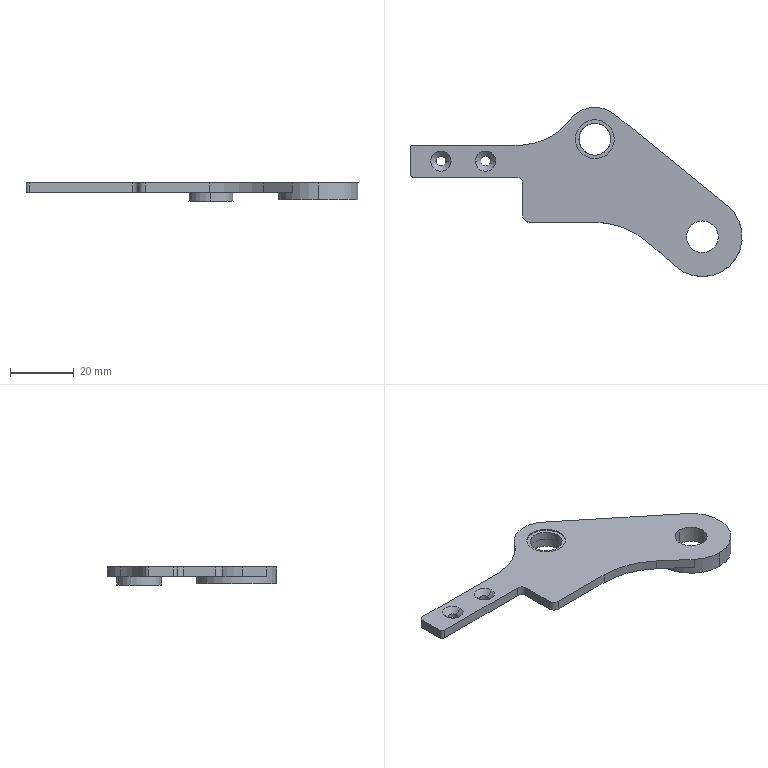Part | NX | features BREP 2, Delete Body 1 | 1 solid | 39 faces | box 104.242 x 53.12 x 5.7 mm | volume 7724 mm3 | cylinder 22 | plane 12 | cone 4 | spline 1 | commonest cylinder face diameters 10 x6 3 x4 2 x2 4 x2 12.2 x2 14 x2
STEP:
#1=CARTESIAN_POINT('',(-175.404,191.172,-0.7));
#2=VERTEX_POINT('',#1);
#3=CARTESIAN_POINT('',(-175.404,201.172,-0.7));
#4=VERTEX_POINT('',#3);
#5=CARTESIAN_POINT('',(-175.404,196.172,-0.7));
#6=DIRECTION('',(0.,0.,-1.));
#7=DIRECTION('',(0.,1.,0.));
#8=AXIS2_PLACEMENT_3D('',#5,#6,#7);
#9=CIRCLE('',#8,5.);
#10=EDGE_CURVE('',#2,#4,#9,.T.);
#11=ORIENTED_EDGE('',*,*,#10,.T.);
#12=CARTESIAN_POINT('',(-175.404,201.172,2.));
#13=VERTEX_POINT('',#12);
#14=CARTESIAN_POINT('',(-175.404,201.172,-17.671));
#15=DIRECTION('',(0.,0.,1.));
#16=VECTOR('',#15,1000.);
#17=LINE('',#14,#16);
#18=EDGE_CURVE('',#13,#4,#17,.F.);
#19=ORIENTED_EDGE('',*,*,#18,.F.);
#20=CARTESIAN_POINT('',(-176.152,201.116,2.));
#21=VERTEX_POINT('',#20);
#22=CARTESIAN_POINT('',(-175.404,201.172,2.));
#23=CARTESIAN_POINT('',(-175.654,201.172,2.));
#24=CARTESIAN_POINT('',(-175.904,201.153,2.));
#25=CARTESIAN_POINT('',(-176.152,201.116,2.));
#26=B_SPLINE_CURVE_WITH_KNOTS('',3,(#22,#23,#24,#25),.UNSPECIFIED.,.F.,.F.,(4,4),(0.,1.),.UNSPECIFIED.);
#27=EDGE_CURVE('',#21,#13,#26,.F.);
#28=ORIENTED_EDGE('',*,*,#27,.F.);
#29=CARTESIAN_POINT('',(-180.403,196.114,2.));
#30=VERTEX_POINT('',#29);
#31=CARTESIAN_POINT('',(-176.152,201.116,2.));
#32=CARTESIAN_POINT('',(-177.332,200.937,2.));
#33=CARTESIAN_POINT('',(-179.552,199.698,2.));
#34=CARTESIAN_POINT('',(-180.417,197.307,2.));
#35=CARTESIAN_POINT('',(-180.403,196.114,2.));
#36=B_SPLINE_CURVE_WITH_KNOTS('',3,(#31,#32,#33,#34,#35),.UNSPECIFIED.,.F.,.F.,(4,1,4),(0.,0.5,1.),.UNSPECIFIED.);
#37=EDGE_CURVE('',#30,#21,#36,.F.);
#38=ORIENTED_EDGE('',*,*,#37,.F.);
#39=CARTESIAN_POINT('',(-175.404,191.172,2.));
#40=VERTEX_POINT('',#39);
#41=CARTESIAN_POINT('',(-180.403,196.114,2.));
#42=CARTESIAN_POINT('',(-180.388,194.815,2.));
#43=CARTESIAN_POINT('',(-179.292,192.239,2.));
#44=CARTESIAN_POINT('',(-176.703,191.172,2.));
#45=CARTESIAN_POINT('',(-175.404,191.172,2.));
#46=B_SPLINE_CURVE_WITH_KNOTS('',3,(#41,#42,#43,#44,#45),.UNSPECIFIED.,.F.,.F.,(4,1,4),(0.,0.5,1.),.UNSPECIFIED.);
#47=EDGE_CURVE('',#40,#30,#46,.F.);
#48=ORIENTED_EDGE('',*,*,#47,.F.);
#49=CARTESIAN_POINT('',(-175.404,191.172,-17.671));
#50=DIRECTION('',(0.,0.,1.));
#51=VECTOR('',#50,1000.);
#52=LINE('',#49,#51);
#53=EDGE_CURVE('',#40,#2,#52,.F.);
#54=ORIENTED_EDGE('',*,*,#53,.T.);
#55=EDGE_LOOP('',(#11,#19,#28,#38,#48,#54));
#56=FACE_BOUND('',#55,.T.);
#57=CARTESIAN_POINT('',(-175.404,196.172,-17.671));
#58=DIRECTION('',(0.,0.,1.));
#59=DIRECTION('',(0.,1.,0.));
#60=AXIS2_PLACEMENT_3D('',#57,#58,#59);
#61=CYLINDRICAL_SURFACE('',#60,5.);
#62=ADVANCED_FACE('',(#56),#61,.F.);
#63=CARTESIAN_POINT('',(-175.404,203.172,-0.7));
#64=VERTEX_POINT('',#63);
#65=CARTESIAN_POINT('',(-175.404,189.172,-0.7));
#66=VERTEX_POINT('',#65);
#67=CARTESIAN_POINT('',(-175.404,196.172,-0.7));
#68=DIRECTION('',(0.,0.,-1.));
#69=DIRECTION('',(0.,1.,0.));
#70=AXIS2_PLACEMENT_3D('',#67,#68,#69);
#71=CIRCLE('',#70,7.);
#72=EDGE_CURVE('',#64,#66,#71,.T.);
#73=ORIENTED_EDGE('',*,*,#72,.F.);
#74=CARTESIAN_POINT('',(-175.404,203.172,2.));
#75=VERTEX_POINT('',#74);
#76=CARTESIAN_POINT('',(-175.404,203.172,-17.671));
#77=DIRECTION('',(0.,0.,1.));
#78=VECTOR('',#77,1000.);
#79=LINE('',#76,#78);
#80=EDGE_CURVE('',#75,#64,#79,.F.);
#81=ORIENTED_EDGE('',*,*,#80,.F.);
#82=CARTESIAN_POINT('',(-175.404,189.172,2.));
#83=VERTEX_POINT('',#82);
#84=CARTESIAN_POINT('',(-175.404,196.172,2.));
#85=DIRECTION('',(0.,0.,-1.));
#86=DIRECTION('',(0.,1.,0.));
#87=AXIS2_PLACEMENT_3D('',#84,#85,#86);
#88=CIRCLE('',#87,7.);
#89=EDGE_CURVE('',#75,#83,#88,.T.);
#90=ORIENTED_EDGE('',*,*,#89,.T.);
#91=CARTESIAN_POINT('',(-175.404,189.172,-17.671));
#92=DIRECTION('',(0.,0.,1.));
#93=VECTOR('',#92,1000.);
#94=LINE('',#91,#93);
#95=EDGE_CURVE('',#83,#66,#94,.F.);
#96=ORIENTED_EDGE('',*,*,#95,.T.);
#97=EDGE_LOOP('',(#73,#81,#90,#96));
#98=FACE_BOUND('',#97,.T.);
#99=CARTESIAN_POINT('',(-175.404,196.172,-17.671));
#100=DIRECTION('',(0.,0.,1.));
#101=DIRECTION('',(0.,1.,0.));
#102=AXIS2_PLACEMENT_3D('',#99,#100,#101);
#103=CYLINDRICAL_SURFACE('',#102,7.);
#104=ADVANCED_FACE('',(#98),#103,.T.);
#105=CARTESIAN_POINT('',(-141.672,178.052,-0.3));
#106=VERTEX_POINT('',#105);
#107=CARTESIAN_POINT('',(-141.672,153.052,-0.3));
#108=VERTEX_POINT('',#107);
#109=CARTESIAN_POINT('',(-141.672,165.552,-0.3));
#110=DIRECTION('',(0.,0.,-1.));
#111=DIRECTION('',(0.,1.,0.));
#112=AXIS2_PLACEMENT_3D('',#109,#110,#111);
#113=CIRCLE('',#112,12.5);
#114=EDGE_CURVE('',#106,#108,#113,.T.);
#115=ORIENTED_EDGE('',*,*,#114,.F.);
#116=CARTESIAN_POINT('',(-141.672,178.052,2.));
#117=VERTEX_POINT('',#116);
#118=CARTESIAN_POINT('',(-141.672,178.052,2.));
#119=DIRECTION('',(0.,0.,1.));
#120=VECTOR('',#119,1000.);
#121=LINE('',#118,#120);
#122=EDGE_CURVE('',#117,#106,#121,.F.);
#123=ORIENTED_EDGE('',*,*,#122,.F.);
#124=CARTESIAN_POINT('',(-133.791,175.255,2.));
#125=VERTEX_POINT('',#124);
#126=CARTESIAN_POINT('',(-141.672,165.552,2.));
#127=DIRECTION('',(0.,0.,-1.));
#128=DIRECTION('',(0.,1.,0.));
#129=AXIS2_PLACEMENT_3D('',#126,#127,#128);
#130=CIRCLE('',#129,12.5);
#131=EDGE_CURVE('',#117,#125,#130,.T.);
#132=ORIENTED_EDGE('',*,*,#131,.T.);
#133=CARTESIAN_POINT('',(-133.791,175.255,5.));
#134=VERTEX_POINT('',#133);
#135=CARTESIAN_POINT('',(-133.791,175.255,2.));
#136=DIRECTION('',(0.,0.,1.));
#137=VECTOR('',#136,1000.);
#138=LINE('',#135,#137);
#139=EDGE_CURVE('',#125,#134,#138,.T.);
#140=ORIENTED_EDGE('',*,*,#139,.T.);
#141=CARTESIAN_POINT('',(-141.672,153.052,5.));
#142=VERTEX_POINT('',#141);
#143=CARTESIAN_POINT('',(-141.672,165.552,5.));
#144=DIRECTION('',(0.,0.,-1.));
#145=DIRECTION('',(0.,1.,0.));
#146=AXIS2_PLACEMENT_3D('',#143,#144,#145);
#147=CIRCLE('',#146,12.5);
#148=EDGE_CURVE('',#134,#142,#147,.T.);
#149=ORIENTED_EDGE('',*,*,#148,.T.);
#150=CARTESIAN_POINT('',(-141.672,153.052,2.));
#151=DIRECTION('',(0.,0.,1.));
#152=VECTOR('',#151,1000.);
#153=LINE('',#150,#152);
#154=EDGE_CURVE('',#142,#108,#153,.F.);
#155=ORIENTED_EDGE('',*,*,#154,.T.);
#156=EDGE_LOOP('',(#115,#123,#132,#140,#149,#155));
#157=FACE_BOUND('',#156,.T.);
#158=CARTESIAN_POINT('',(-141.672,165.552,2.));
#159=DIRECTION('',(0.,0.,1.));
#160=DIRECTION('',(0.,1.,0.));
#161=AXIS2_PLACEMENT_3D('',#158,#159,#160);
#162=CYLINDRICAL_SURFACE('',#161,12.5);
#163=ADVANCED_FACE('',(#157),#162,.T.);
#164=CARTESIAN_POINT('',(-208.209,189.293,2.));
#165=VERTEX_POINT('',#164);
#166=CARTESIAN_POINT('',(-211.209,189.293,2.));
#167=VERTEX_POINT('',#166);
#168=CARTESIAN_POINT('',(-209.709,189.293,2.));
#169=DIRECTION('',(0.,0.,-1.));
#170=DIRECTION('',(0.,1.,0.));
#171=AXIS2_PLACEMENT_3D('',#168,#169,#170);
#172=CIRCLE('',#171,1.5);
#173=EDGE_CURVE('',#165,#167,#172,.T.);
#174=ORIENTED_EDGE('',*,*,#173,.T.);
#175=CARTESIAN_POINT('',(-211.209,189.293,3.3));
#176=VERTEX_POINT('',#175);
#177=CARTESIAN_POINT('',(-211.209,189.293,-0.5));
#178=DIRECTION('',(0.,0.,1.));
#179=VECTOR('',#178,1000.);
#180=LINE('',#177,#179);
#181=EDGE_CURVE('',#167,#176,#180,.T.);
#182=ORIENTED_EDGE('',*,*,#181,.T.);
#183=CARTESIAN_POINT('',(-208.209,189.293,3.3));
#184=VERTEX_POINT('',#183);
#185=CARTESIAN_POINT('',(-209.709,189.293,3.3));
#186=DIRECTION('',(0.,0.,1.));
#187=DIRECTION('',(-1.,0.,0.));
#188=AXIS2_PLACEMENT_3D('',#185,#186,#187);
#189=CIRCLE('',#188,1.5);
#190=EDGE_CURVE('',#176,#184,#189,.T.);
#191=ORIENTED_EDGE('',*,*,#190,.T.);
#192=CARTESIAN_POINT('',(-208.209,189.293,-0.5));
#193=DIRECTION('',(0.,0.,1.));
#194=VECTOR('',#193,1000.);
#195=LINE('',#192,#194);
#196=EDGE_CURVE('',#165,#184,#195,.T.);
#197=ORIENTED_EDGE('',*,*,#196,.F.);
#198=EDGE_LOOP('',(#174,#182,#191,#197));
#199=FACE_BOUND('',#198,.T.);
#200=CARTESIAN_POINT('',(-209.709,189.293,-0.5));
#201=DIRECTION('',(0.,0.,1.));
#202=DIRECTION('',(-1.,0.,0.));
#203=AXIS2_PLACEMENT_3D('',#200,#201,#202);
#204=CYLINDRICAL_SURFACE('',#203,1.5);
#205=ADVANCED_FACE('',(#199),#204,.F.);
#206=CARTESIAN_POINT('',(-222.209,189.293,2.));
#207=VERTEX_POINT('',#206);
#208=CARTESIAN_POINT('',(-225.209,189.293,2.));
#209=VERTEX_POINT('',#208);
#210=CARTESIAN_POINT('',(-223.709,189.293,2.));
#211=DIRECTION('',(0.,0.,-1.));
#212=DIRECTION('',(0.,1.,0.));
#213=AXIS2_PLACEMENT_3D('',#210,#211,#212);
#214=CIRCLE('',#213,1.5);
#215=EDGE_CURVE('',#207,#209,#214,.T.);
#216=ORIENTED_EDGE('',*,*,#215,.T.);
#217=CARTESIAN_POINT('',(-225.209,189.293,3.3));
#218=VERTEX_POINT('',#217);
#219=CARTESIAN_POINT('',(-225.209,189.293,-0.5));
#220=DIRECTION('',(0.,0.,1.));
#221=VECTOR('',#220,1000.);
#222=LINE('',#219,#221);
#223=EDGE_CURVE('',#209,#218,#222,.T.);
#224=ORIENTED_EDGE('',*,*,#223,.T.);
#225=CARTESIAN_POINT('',(-222.209,189.293,3.3));
#226=VERTEX_POINT('',#225);
#227=CARTESIAN_POINT('',(-223.709,189.293,3.3));
#228=DIRECTION('',(0.,0.,1.));
#229=DIRECTION('',(-1.,0.,0.));
#230=AXIS2_PLACEMENT_3D('',#227,#228,#229);
#231=CIRCLE('',#230,1.5);
#232=EDGE_CURVE('',#218,#226,#231,.T.);
#233=ORIENTED_EDGE('',*,*,#232,.T.);
#234=CARTESIAN_POINT('',(-222.209,189.293,-0.5));
#235=DIRECTION('',(0.,0.,1.));
#236=VECTOR('',#235,1000.);
#237=LINE('',#234,#236);
#238=EDGE_CURVE('',#207,#226,#237,.T.);
#239=ORIENTED_EDGE('',*,*,#238,.F.);
#240=EDGE_LOOP('',(#216,#224,#233,#239));
#241=FACE_BOUND('',#240,.T.);
#242=CARTESIAN_POINT('',(-223.709,189.293,-0.5));
#243=DIRECTION('',(0.,0.,1.));
#244=DIRECTION('',(-1.,0.,0.));
#245=AXIS2_PLACEMENT_3D('',#242,#243,#244);
#246=CYLINDRICAL_SURFACE('',#245,1.5);
#247=ADVANCED_FACE('',(#241),#246,.F.);
#248=CARTESIAN_POINT('',(-181.503,196.101,5.));
#249=VERTEX_POINT('',#248);
#250=CARTESIAN_POINT('',(-169.304,196.243,5.));
#251=VERTEX_POINT('',#250);
#252=CARTESIAN_POINT('',(-175.403,196.172,5.));
#253=DIRECTION('',(0.,0.,1.));
#254=DIRECTION('',(0.,1.,0.));
#255=AXIS2_PLACEMENT_3D('',#252,#253,#254);
#256=CIRCLE('',#255,6.1);
#257=EDGE_CURVE('',#249,#251,#256,.T.);
#258=ORIENTED_EDGE('',*,*,#257,.T.);
#259=CARTESIAN_POINT('',(-169.304,196.243,4.6));
#260=VERTEX_POINT('',#259);
#261=CARTESIAN_POINT('',(-169.304,196.243,2.785));
#262=DIRECTION('',(0.,0.,-1.));
#263=VECTOR('',#262,1000.);
#264=LINE('',#261,#263);
#265=EDGE_CURVE('',#260,#251,#264,.F.);
#266=ORIENTED_EDGE('',*,*,#265,.F.);
#267=CARTESIAN_POINT('',(-181.503,196.101,4.6));
#268=VERTEX_POINT('',#267);
#269=CARTESIAN_POINT('',(-175.403,196.172,4.6));
#270=DIRECTION('',(0.,0.,-1.));
#271=DIRECTION('',(0.,-1.,0.));
#272=AXIS2_PLACEMENT_3D('',#269,#270,#271);
#273=CIRCLE('',#272,6.1);
#274=EDGE_CURVE('',#260,#268,#273,.T.);
#275=ORIENTED_EDGE('',*,*,#274,.T.);
#276=CARTESIAN_POINT('',(-181.503,196.101,2.785));
#277=DIRECTION('',(0.,0.,-1.));
#278=VECTOR('',#277,1000.);
#279=LINE('',#276,#278);
#280=EDGE_CURVE('',#268,#249,#279,.F.);
#281=ORIENTED_EDGE('',*,*,#280,.T.);
#282=EDGE_LOOP('',(#258,#266,#275,#281));
#283=FACE_BOUND('',#282,.T.);
#284=CARTESIAN_POINT('',(-175.403,196.172,2.785));
#285=DIRECTION('',(0.,0.,-1.));
#286=DIRECTION('',(0.9999,0.01167,0.));
#287=AXIS2_PLACEMENT_3D('',#284,#285,#286);
#288=CYLINDRICAL_SURFACE('',#287,6.1);
#289=ADVANCED_FACE('',(#283),#288,.F.);
#290=ORIENTED_EDGE('',*,*,#190,.F.);
#291=CARTESIAN_POINT('',(-212.909,189.293,5.));
#292=VERTEX_POINT('',#291);
#293=CARTESIAN_POINT('',(-211.209,189.293,3.3));
#294=DIRECTION('',(-0.7071,0.,0.7071));
#295=VECTOR('',#294,1000.);
#296=LINE('',#293,#295);
#297=EDGE_CURVE('',#176,#292,#296,.T.);
#298=ORIENTED_EDGE('',*,*,#297,.T.);
#299=CARTESIAN_POINT('',(-206.509,189.293,5.));
#300=VERTEX_POINT('',#299);
#301=CARTESIAN_POINT('',(-209.709,189.293,5.));
#302=DIRECTION('',(0.,0.,-1.));
#303=DIRECTION('',(0.,1.,0.));
#304=AXIS2_PLACEMENT_3D('',#301,#302,#303);
#305=CIRCLE('',#304,3.2);
#306=EDGE_CURVE('',#300,#292,#305,.T.);
#307=ORIENTED_EDGE('',*,*,#306,.F.);
#308=CARTESIAN_POINT('',(-208.209,189.293,3.3));
#309=DIRECTION('',(0.7071,0.,0.7071));
#310=VECTOR('',#309,1000.);
#311=LINE('',#308,#310);
#312=EDGE_CURVE('',#184,#300,#311,.T.);
#313=ORIENTED_EDGE('',*,*,#312,.F.);
#314=EDGE_LOOP('',(#290,#298,#307,#313));
#315=FACE_BOUND('',#314,.T.);
#316=CARTESIAN_POINT('',(-209.709,189.293,3.3));
#317=DIRECTION('',(0.,0.,1.));
#318=DIRECTION('',(-1.,0.,0.));
#319=AXIS2_PLACEMENT_3D('',#316,#317,#318);
#320=CONICAL_SURFACE('',#319,1.5,0.7854);
#321=ADVANCED_FACE('',(#315),#320,.F.);
#322=ORIENTED_EDGE('',*,*,#232,.F.);
#323=CARTESIAN_POINT('',(-226.909,189.293,5.));
#324=VERTEX_POINT('',#323);
#325=CARTESIAN_POINT('',(-225.209,189.293,3.3));
#326=DIRECTION('',(-0.7071,0.,0.7071));
#327=VECTOR('',#326,1000.);
#328=LINE('',#325,#327);
#329=EDGE_CURVE('',#218,#324,#328,.T.);
#330=ORIENTED_EDGE('',*,*,#329,.T.);
#331=CARTESIAN_POINT('',(-220.509,189.293,5.));
#332=VERTEX_POINT('',#331);
#333=CARTESIAN_POINT('',(-223.709,189.293,5.));
#334=DIRECTION('',(0.,0.,-1.));
#335=DIRECTION('',(0.,1.,0.));
#336=AXIS2_PLACEMENT_3D('',#333,#334,#335);
#337=CIRCLE('',#336,3.2);
#338=EDGE_CURVE('',#332,#324,#337,.T.);
#339=ORIENTED_EDGE('',*,*,#338,.F.);
#340=CARTESIAN_POINT('',(-222.209,189.293,3.3));
#341=DIRECTION('',(0.7071,0.,0.7071));
#342=VECTOR('',#341,1000.);
#343=LINE('',#340,#342);
#344=EDGE_CURVE('',#226,#332,#343,.T.);
#345=ORIENTED_EDGE('',*,*,#344,.F.);
#346=EDGE_LOOP('',(#322,#330,#339,#345));
#347=FACE_BOUND('',#346,.T.);
#348=CARTESIAN_POINT('',(-223.709,189.293,3.3));
#349=DIRECTION('',(0.,0.,1.));
#350=DIRECTION('',(-1.,0.,0.));
#351=AXIS2_PLACEMENT_3D('',#348,#349,#350);
#352=CONICAL_SURFACE('',#351,1.5,0.7854);
#353=ADVANCED_FACE('',(#347),#352,.F.);
#354=CARTESIAN_POINT('',(-141.672,160.552,-0.3));
#355=VERTEX_POINT('',#354);
#356=CARTESIAN_POINT('',(-141.672,170.552,-0.3));
#357=VERTEX_POINT('',#356);
#358=CARTESIAN_POINT('',(-141.672,165.552,-0.3));
#359=DIRECTION('',(0.,0.,-1.));
#360=DIRECTION('',(0.,1.,0.));
#361=AXIS2_PLACEMENT_3D('',#358,#359,#360);
#362=CIRCLE('',#361,5.);
#363=EDGE_CURVE('',#355,#357,#362,.T.);
#364=ORIENTED_EDGE('',*,*,#363,.T.);
#365=CARTESIAN_POINT('',(-141.672,170.552,5.));
#366=VERTEX_POINT('',#365);
#367=CARTESIAN_POINT('',(-141.672,170.552,2.));
#368=DIRECTION('',(0.,0.,1.));
#369=VECTOR('',#368,1000.);
#370=LINE('',#367,#369);
#371=EDGE_CURVE('',#366,#357,#370,.F.);
#372=ORIENTED_EDGE('',*,*,#371,.F.);
#373=CARTESIAN_POINT('',(-141.672,160.552,5.));
#374=VERTEX_POINT('',#373);
#375=CARTESIAN_POINT('',(-141.672,165.552,5.));
#376=DIRECTION('',(0.,0.,-1.));
#377=DIRECTION('',(0.,1.,0.));
#378=AXIS2_PLACEMENT_3D('',#375,#376,#377);
#379=CIRCLE('',#378,5.);
#380=EDGE_CURVE('',#374,#366,#379,.T.);
#381=ORIENTED_EDGE('',*,*,#380,.F.);
#382=CARTESIAN_POINT('',(-141.672,160.552,2.));
#383=DIRECTION('',(0.,0.,1.));
#384=VECTOR('',#383,1000.);
#385=LINE('',#382,#384);
#386=EDGE_CURVE('',#374,#355,#385,.F.);
#387=ORIENTED_EDGE('',*,*,#386,.T.);
#388=EDGE_LOOP('',(#364,#372,#381,#387));
#389=FACE_BOUND('',#388,.T.);
#390=CARTESIAN_POINT('',(-141.672,165.552,2.));
#391=DIRECTION('',(0.,0.,1.));
#392=DIRECTION('',(0.,1.,0.));
#393=AXIS2_PLACEMENT_3D('',#390,#391,#392);
#394=CYLINDRICAL_SURFACE('',#393,5.);
#395=ADVANCED_FACE('',(#389),#394,.F.);
#396=CARTESIAN_POINT('',(-180.403,196.114,4.6));
#397=VERTEX_POINT('',#396);
#398=CARTESIAN_POINT('',(-170.403,196.231,4.6));
#399=VERTEX_POINT('',#398);
#400=CARTESIAN_POINT('',(-175.403,196.172,4.6));
#401=DIRECTION('',(0.,0.,1.));
#402=DIRECTION('',(0.,-1.,0.));
#403=AXIS2_PLACEMENT_3D('',#400,#401,#402);
#404=CIRCLE('',#403,5.);
#405=EDGE_CURVE('',#397,#399,#404,.T.);
#406=ORIENTED_EDGE('',*,*,#405,.T.);
#407=CARTESIAN_POINT('',(-170.404,196.231,2.));
#408=VERTEX_POINT('',#407);
#409=CARTESIAN_POINT('',(-170.403,196.231,2.785));
#410=DIRECTION('',(0.,0.,-1.));
#411=VECTOR('',#410,1000.);
#412=LINE('',#409,#411);
#413=EDGE_CURVE('',#408,#399,#412,.F.);
#414=ORIENTED_EDGE('',*,*,#413,.F.);
#415=CARTESIAN_POINT('',(-174.655,191.228,2.));
#416=VERTEX_POINT('',#415);
#417=CARTESIAN_POINT('',(-170.403,196.231,2.));
#418=CARTESIAN_POINT('',(-170.39,195.037,2.));
#419=CARTESIAN_POINT('',(-171.254,192.646,2.));
#420=CARTESIAN_POINT('',(-173.475,191.407,2.));
#421=CARTESIAN_POINT('',(-174.655,191.228,2.));
#422=B_SPLINE_CURVE_WITH_KNOTS('',3,(#417,#418,#419,#420,#421),.UNSPECIFIED.,.F.,.F.,(4,1,4),(0.,0.5,1.),.UNSPECIFIED.);
#423=EDGE_CURVE('',#408,#416,#422,.T.);
#424=ORIENTED_EDGE('',*,*,#423,.T.);
#425=CARTESIAN_POINT('',(-174.655,191.228,2.));
#426=CARTESIAN_POINT('',(-174.903,191.191,2.));
#427=CARTESIAN_POINT('',(-175.153,191.172,2.));
#428=CARTESIAN_POINT('',(-175.404,191.172,2.));
#429=B_SPLINE_CURVE_WITH_KNOTS('',3,(#425,#426,#427,#428),.UNSPECIFIED.,.F.,.F.,(4,4),(0.,1.),.UNSPECIFIED.);
#430=EDGE_CURVE('',#416,#40,#429,.T.);
#431=ORIENTED_EDGE('',*,*,#430,.T.);
#432=ORIENTED_EDGE('',*,*,#47,.T.);
#433=CARTESIAN_POINT('',(-180.403,196.114,2.785));
#434=DIRECTION('',(0.,0.,-1.));
#435=VECTOR('',#434,1000.);
#436=LINE('',#433,#435);
#437=EDGE_CURVE('',#30,#397,#436,.F.);
#438=ORIENTED_EDGE('',*,*,#437,.T.);
#439=EDGE_LOOP('',(#406,#414,#424,#431,#432,#438));
#440=FACE_BOUND('',#439,.T.);
#441=CARTESIAN_POINT('',(-175.403,196.172,2.785));
#442=DIRECTION('',(0.,0.,-1.));
#443=DIRECTION('',(0.9999,0.01167,0.));
#444=AXIS2_PLACEMENT_3D('',#441,#442,#443);
#445=CYLINDRICAL_SURFACE('',#444,5.);
#446=ADVANCED_FACE('',(#440),#445,.F.);
#447=ORIENTED_EDGE('',*,*,#413,.T.);
#448=CARTESIAN_POINT('',(-175.403,196.172,4.6));
#449=DIRECTION('',(0.,0.,1.));
#450=DIRECTION('',(0.,-1.,0.));
#451=AXIS2_PLACEMENT_3D('',#448,#449,#450);
#452=CIRCLE('',#451,5.);
#453=EDGE_CURVE('',#399,#397,#452,.T.);
#454=ORIENTED_EDGE('',*,*,#453,.T.);
#455=ORIENTED_EDGE('',*,*,#437,.F.);
#456=ORIENTED_EDGE('',*,*,#37,.T.);
#457=ORIENTED_EDGE('',*,*,#27,.T.);
#458=CARTESIAN_POINT('',(-175.404,201.172,2.));
#459=CARTESIAN_POINT('',(-174.104,201.172,2.));
#460=CARTESIAN_POINT('',(-171.515,200.106,2.));
#461=CARTESIAN_POINT('',(-170.419,197.53,2.));
#462=CARTESIAN_POINT('',(-170.403,196.231,2.));
#463=B_SPLINE_CURVE_WITH_KNOTS('',3,(#458,#459,#460,#461,#462),.UNSPECIFIED.,.F.,.F.,(4,1,4),(0.,0.5,1.),.UNSPECIFIED.);
#464=EDGE_CURVE('',#13,#408,#463,.T.);
#465=ORIENTED_EDGE('',*,*,#464,.T.);
#466=EDGE_LOOP('',(#447,#454,#455,#456,#457,#465));
#467=FACE_BOUND('',#466,.T.);
#468=CARTESIAN_POINT('',(-175.403,196.172,2.785));
#469=DIRECTION('',(0.,0.,-1.));
#470=DIRECTION('',(0.9999,0.01167,0.));
#471=AXIS2_PLACEMENT_3D('',#468,#469,#470);
#472=CYLINDRICAL_SURFACE('',#471,5.);
#473=ADVANCED_FACE('',(#467),#472,.F.);
#474=ORIENTED_EDGE('',*,*,#371,.T.);
#475=CARTESIAN_POINT('',(-141.672,165.552,-0.3));
#476=DIRECTION('',(0.,0.,-1.));
#477=DIRECTION('',(0.,1.,0.));
#478=AXIS2_PLACEMENT_3D('',#475,#476,#477);
#479=CIRCLE('',#478,5.);
#480=EDGE_CURVE('',#357,#355,#479,.T.);
#481=ORIENTED_EDGE('',*,*,#480,.T.);
#482=ORIENTED_EDGE('',*,*,#386,.F.);
#483=CARTESIAN_POINT('',(-141.672,165.552,5.));
#484=DIRECTION('',(0.,0.,-1.));
#485=DIRECTION('',(0.,1.,0.));
#486=AXIS2_PLACEMENT_3D('',#483,#484,#485);
#487=CIRCLE('',#486,5.);
#488=EDGE_CURVE('',#366,#374,#487,.T.);
#489=ORIENTED_EDGE('',*,*,#488,.F.);
#490=EDGE_LOOP('',(#474,#481,#482,#489));
#491=FACE_BOUND('',#490,.T.);
#492=CARTESIAN_POINT('',(-141.672,165.552,2.));
#493=DIRECTION('',(0.,0.,1.));
#494=DIRECTION('',(0.,1.,0.));
#495=AXIS2_PLACEMENT_3D('',#492,#493,#494);
#496=CYLINDRICAL_SURFACE('',#495,5.);
#497=ADVANCED_FACE('',(#491),#496,.F.);
#498=ORIENTED_EDGE('',*,*,#329,.F.);
#499=CARTESIAN_POINT('',(-223.709,189.293,3.3));
#500=DIRECTION('',(0.,0.,1.));
#501=DIRECTION('',(-1.,0.,0.));
#502=AXIS2_PLACEMENT_3D('',#499,#500,#501);
#503=CIRCLE('',#502,1.5);
#504=EDGE_CURVE('',#226,#218,#503,.T.);
#505=ORIENTED_EDGE('',*,*,#504,.F.);
#506=ORIENTED_EDGE('',*,*,#344,.T.);
#507=CARTESIAN_POINT('',(-223.709,189.293,5.));
#508=DIRECTION('',(0.,0.,-1.));
#509=DIRECTION('',(0.,1.,0.));
#510=AXIS2_PLACEMENT_3D('',#507,#508,#509);
#511=CIRCLE('',#510,3.2);
#512=EDGE_CURVE('',#324,#332,#511,.T.);
#513=ORIENTED_EDGE('',*,*,#512,.F.);
#514=EDGE_LOOP('',(#498,#505,#506,#513));
#515=FACE_BOUND('',#514,.T.);
#516=CARTESIAN_POINT('',(-223.709,189.293,3.3));
#517=DIRECTION('',(0.,0.,1.));
#518=DIRECTION('',(-1.,0.,0.));
#519=AXIS2_PLACEMENT_3D('',#516,#517,#518);
#520=CONICAL_SURFACE('',#519,1.5,0.7854);
#521=ADVANCED_FACE('',(#515),#520,.F.);
#522=ORIENTED_EDGE('',*,*,#297,.F.);
#523=CARTESIAN_POINT('',(-209.709,189.293,3.3));
#524=DIRECTION('',(0.,0.,1.));
#525=DIRECTION('',(-1.,0.,0.));
#526=AXIS2_PLACEMENT_3D('',#523,#524,#525);
#527=CIRCLE('',#526,1.5);
#528=EDGE_CURVE('',#184,#176,#527,.T.);
#529=ORIENTED_EDGE('',*,*,#528,.F.);
#530=ORIENTED_EDGE('',*,*,#312,.T.);
#531=CARTESIAN_POINT('',(-209.709,189.293,5.));
#532=DIRECTION('',(0.,0.,-1.));
#533=DIRECTION('',(0.,1.,0.));
#534=AXIS2_PLACEMENT_3D('',#531,#532,#533);
#535=CIRCLE('',#534,3.2);
#536=EDGE_CURVE('',#292,#300,#535,.T.);
#537=ORIENTED_EDGE('',*,*,#536,.F.);
#538=EDGE_LOOP('',(#522,#529,#530,#537));
#539=FACE_BOUND('',#538,.T.);
#540=CARTESIAN_POINT('',(-209.709,189.293,3.3));
#541=DIRECTION('',(0.,0.,1.));
#542=DIRECTION('',(-1.,0.,0.));
#543=AXIS2_PLACEMENT_3D('',#540,#541,#542);
#544=CONICAL_SURFACE('',#543,1.5,0.7854);
#545=ADVANCED_FACE('',(#539),#544,.F.);
#546=CARTESIAN_POINT('',(-141.672,165.552,-0.3));
#547=DIRECTION('',(0.,0.,-1.));
#548=DIRECTION('',(0.,1.,0.));
#549=AXIS2_PLACEMENT_3D('',#546,#547,#548);
#550=CIRCLE('',#549,12.5);
#551=EDGE_CURVE('',#108,#106,#550,.T.);
#552=ORIENTED_EDGE('',*,*,#551,.T.);
#553=ORIENTED_EDGE('',*,*,#114,.T.);
#554=EDGE_LOOP('',(#552,#553));
#555=FACE_BOUND('',#554,.T.);
#556=ORIENTED_EDGE('',*,*,#363,.F.);
#557=ORIENTED_EDGE('',*,*,#480,.F.);
#558=EDGE_LOOP('',(#556,#557));
#559=FACE_BOUND('',#558,.T.);
#560=CARTESIAN_POINT('',(-146.593,163.872,-0.3));
#561=DIRECTION('',(0.,0.,-1.));
#562=DIRECTION('',(1.,0.,0.));
#563=AXIS2_PLACEMENT_3D('',#560,#561,#562);
#564=PLANE('',#563);
#565=ADVANCED_FACE('',(#555,#559),#564,.T.);
#566=ORIENTED_EDGE('',*,*,#265,.T.);
#567=CARTESIAN_POINT('',(-175.403,196.172,5.));
#568=DIRECTION('',(0.,0.,1.));
#569=DIRECTION('',(0.,1.,0.));
#570=AXIS2_PLACEMENT_3D('',#567,#568,#569);
#571=CIRCLE('',#570,6.1);
#572=EDGE_CURVE('',#251,#249,#571,.T.);
#573=ORIENTED_EDGE('',*,*,#572,.T.);
#574=ORIENTED_EDGE('',*,*,#280,.F.);
#575=CARTESIAN_POINT('',(-175.403,196.172,4.6));
#576=DIRECTION('',(0.,0.,-1.));
#577=DIRECTION('',(0.,-1.,0.));
#578=AXIS2_PLACEMENT_3D('',#575,#576,#577);
#579=CIRCLE('',#578,6.1);
#580=EDGE_CURVE('',#268,#260,#579,.T.);
#581=ORIENTED_EDGE('',*,*,#580,.T.);
#582=EDGE_LOOP('',(#566,#573,#574,#581));
#583=FACE_BOUND('',#582,.T.);
#584=CARTESIAN_POINT('',(-175.403,196.172,2.785));
#585=DIRECTION('',(0.,0.,-1.));
#586=DIRECTION('',(0.9999,0.01167,0.));
#587=AXIS2_PLACEMENT_3D('',#584,#585,#586);
#588=CYLINDRICAL_SURFACE('',#587,6.1);
#589=ADVANCED_FACE('',(#583),#588,.F.);
#590=ORIENTED_EDGE('',*,*,#580,.F.);
#591=ORIENTED_EDGE('',*,*,#274,.F.);
#592=EDGE_LOOP('',(#590,#591));
#593=FACE_BOUND('',#592,.T.);
#594=ORIENTED_EDGE('',*,*,#405,.F.);
#595=ORIENTED_EDGE('',*,*,#453,.F.);
#596=EDGE_LOOP('',(#594,#595));
#597=FACE_BOUND('',#596,.T.);
#598=CARTESIAN_POINT('',(-175.464,201.372,4.6));
#599=DIRECTION('',(0.,0.,1.));
#600=DIRECTION('',(-1.,0.,0.));
#601=AXIS2_PLACEMENT_3D('',#598,#599,#600);
#602=PLANE('',#601);
#603=ADVANCED_FACE('',(#593,#597),#602,.T.);
#604=CARTESIAN_POINT('',(-169.098,203.934,5.));
#605=VERTEX_POINT('',#604);
#606=CARTESIAN_POINT('',(32.582,40.112,5.));
#607=DIRECTION('',(-0.7762,0.6305,0.));
#608=VECTOR('',#607,1000.);
#609=LINE('',#606,#608);
#610=EDGE_CURVE('',#134,#605,#609,.T.);
#611=ORIENTED_EDGE('',*,*,#610,.T.);
#612=CARTESIAN_POINT('',(-183.399,202.177,5.));
#613=VERTEX_POINT('',#612);
#614=CARTESIAN_POINT('',(-175.403,196.172,5.));
#615=DIRECTION('',(0.,0.,1.));
#616=DIRECTION('',(1.,0.,0.));
#617=AXIS2_PLACEMENT_3D('',#614,#615,#616);
#618=CIRCLE('',#617,10.);
#619=EDGE_CURVE('',#605,#613,#618,.T.);
#620=ORIENTED_EDGE('',*,*,#619,.T.);
#621=CARTESIAN_POINT('',(-198.567,194.293,5.));
#622=VERTEX_POINT('',#621);
#623=CARTESIAN_POINT('',(-198.567,194.293,5.));
#624=CARTESIAN_POINT('',(-188.816,194.965,5.));
#625=CARTESIAN_POINT('',(-183.399,202.177,5.));
#626=B_SPLINE_CURVE_WITH_KNOTS('',2,(#623,#624,#625),.UNSPECIFIED.,.F.,.F.,(3,3),(0.,1.),.PIECEWISE_BEZIER_KNOTS.);
#627=EDGE_CURVE('',#622,#613,#626,.T.);
#628=ORIENTED_EDGE('',*,*,#627,.F.);
#629=CARTESIAN_POINT('',(-232.414,194.293,5.));
#630=VERTEX_POINT('',#629);
#631=CARTESIAN_POINT('',(-214.519,194.293,5.));
#632=DIRECTION('',(1.,0.,0.));
#633=VECTOR('',#632,1000.);
#634=LINE('',#631,#633);
#635=EDGE_CURVE('',#630,#622,#634,.T.);
#636=ORIENTED_EDGE('',*,*,#635,.F.);
#637=CARTESIAN_POINT('',(-233.414,193.293,5.));
#638=VERTEX_POINT('',#637);
#639=CARTESIAN_POINT('',(-232.414,193.293,5.));
#640=DIRECTION('',(0.,0.,1.));
#641=DIRECTION('',(0.,1.,0.));
#642=AXIS2_PLACEMENT_3D('',#639,#640,#641);
#643=CIRCLE('',#642,1.);
#644=EDGE_CURVE('',#630,#638,#643,.T.);
#645=ORIENTED_EDGE('',*,*,#644,.T.);
#646=CARTESIAN_POINT('',(-233.414,185.293,5.));
#647=VERTEX_POINT('',#646);
#648=CARTESIAN_POINT('',(-233.414,185.793,5.));
#649=DIRECTION('',(0.,-1.,0.));
#650=VECTOR('',#649,1000.);
#651=LINE('',#648,#650);
#652=EDGE_CURVE('',#638,#647,#651,.T.);
#653=ORIENTED_EDGE('',*,*,#652,.T.);
#654=CARTESIAN_POINT('',(-232.414,184.293,5.));
#655=VERTEX_POINT('',#654);
#656=CARTESIAN_POINT('',(-232.414,185.293,5.));
#657=DIRECTION('',(0.,0.,1.));
#658=DIRECTION('',(0.,1.,0.));
#659=AXIS2_PLACEMENT_3D('',#656,#657,#658);
#660=CIRCLE('',#659,1.);
#661=EDGE_CURVE('',#647,#655,#660,.T.);
#662=ORIENTED_EDGE('',*,*,#661,.T.);
#663=CARTESIAN_POINT('',(-200.068,184.293,5.));
#664=VERTEX_POINT('',#663);
#665=CARTESIAN_POINT('',(-141.672,184.293,5.));
#666=DIRECTION('',(1.,0.,0.));
#667=VECTOR('',#666,1000.);
#668=LINE('',#665,#667);
#669=EDGE_CURVE('',#655,#664,#668,.T.);
#670=ORIENTED_EDGE('',*,*,#669,.T.);
#671=CARTESIAN_POINT('',(-198.068,182.293,5.));
#672=VERTEX_POINT('',#671);
#673=CARTESIAN_POINT('',(-200.068,182.293,5.));
#674=DIRECTION('',(0.,0.,-1.));
#675=DIRECTION('',(0.,1.,0.));
#676=AXIS2_PLACEMENT_3D('',#673,#674,#675);
#677=CIRCLE('',#676,2.);
#678=EDGE_CURVE('',#664,#672,#677,.T.);
#679=ORIENTED_EDGE('',*,*,#678,.T.);
#680=CARTESIAN_POINT('',(-198.068,172.145,5.));
#681=VERTEX_POINT('',#680);
#682=CARTESIAN_POINT('',(-198.068,170.145,5.));
#683=DIRECTION('',(0.,-1.,0.));
#684=VECTOR('',#683,1000.);
#685=LINE('',#682,#684);
#686=EDGE_CURVE('',#672,#681,#685,.T.);
#687=ORIENTED_EDGE('',*,*,#686,.T.);
#688=CARTESIAN_POINT('',(-196.068,170.145,5.));
#689=VERTEX_POINT('',#688);
#690=CARTESIAN_POINT('',(-196.068,172.145,5.));
#691=DIRECTION('',(0.,0.,1.));
#692=DIRECTION('',(0.,1.,0.));
#693=AXIS2_PLACEMENT_3D('',#690,#691,#692);
#694=CIRCLE('',#693,2.);
#695=EDGE_CURVE('',#681,#689,#694,.T.);
#696=ORIENTED_EDGE('',*,*,#695,.T.);
#697=CARTESIAN_POINT('',(-175.761,170.145,5.));
#698=VERTEX_POINT('',#697);
#699=CARTESIAN_POINT('',(-175.761,170.145,5.));
#700=DIRECTION('',(1.,0.,0.));
#701=VECTOR('',#700,1000.);
#702=LINE('',#699,#701);
#703=EDGE_CURVE('',#689,#698,#702,.T.);
#704=ORIENTED_EDGE('',*,*,#703,.T.);
#705=CARTESIAN_POINT('',(-158.769,163.815,5.));
#706=VERTEX_POINT('',#705);
#707=CARTESIAN_POINT('',(-175.761,144.174,5.));
#708=DIRECTION('',(0.,0.,-1.));
#709=DIRECTION('',(1.,0.,0.));
#710=AXIS2_PLACEMENT_3D('',#707,#708,#709);
#711=CIRCLE('',#710,25.971);
#712=EDGE_CURVE('',#698,#706,#711,.T.);
#713=ORIENTED_EDGE('',*,*,#712,.T.);
#714=CARTESIAN_POINT('',(-149.851,156.099,5.));
#715=VERTEX_POINT('',#714);
#716=CARTESIAN_POINT('',(-149.851,156.099,5.));
#717=DIRECTION('',(-0.7563,0.6543,0.));
#718=VECTOR('',#717,1000.);
#719=LINE('',#716,#718);
#720=EDGE_CURVE('',#715,#706,#719,.T.);
#721=ORIENTED_EDGE('',*,*,#720,.F.);
#722=CARTESIAN_POINT('',(-141.672,165.552,5.));
#723=DIRECTION('',(0.,0.,-1.));
#724=DIRECTION('',(0.,1.,0.));
#725=AXIS2_PLACEMENT_3D('',#722,#723,#724);
#726=CIRCLE('',#725,12.5);
#727=EDGE_CURVE('',#142,#715,#726,.T.);
#728=ORIENTED_EDGE('',*,*,#727,.F.);
#729=ORIENTED_EDGE('',*,*,#148,.F.);
#730=EDGE_LOOP('',(#611,#620,#628,#636,#645,#653,#662,#670,#679,#687,#696,#704,#713,#721,#728,#729));
#731=FACE_BOUND('',#730,.T.);
#732=ORIENTED_EDGE('',*,*,#380,.T.);
#733=ORIENTED_EDGE('',*,*,#488,.T.);
#734=EDGE_LOOP('',(#732,#733));
#735=FACE_BOUND('',#734,.T.);
#736=ORIENTED_EDGE('',*,*,#306,.T.);
#737=ORIENTED_EDGE('',*,*,#536,.T.);
#738=EDGE_LOOP('',(#736,#737));
#739=FACE_BOUND('',#738,.T.);
#740=ORIENTED_EDGE('',*,*,#338,.T.);
#741=ORIENTED_EDGE('',*,*,#512,.T.);
#742=EDGE_LOOP('',(#740,#741));
#743=FACE_BOUND('',#742,.T.);
#744=ORIENTED_EDGE('',*,*,#257,.F.);
#745=ORIENTED_EDGE('',*,*,#572,.F.);
#746=EDGE_LOOP('',(#744,#745));
#747=FACE_BOUND('',#746,.T.);
#748=CARTESIAN_POINT('',(-141.672,165.552,5.));
#749=DIRECTION('',(0.,0.,-1.));
#750=DIRECTION('',(1.,0.,0.));
#751=AXIS2_PLACEMENT_3D('',#748,#749,#750);
#752=PLANE('',#751);
#753=ADVANCED_FACE('',(#731,#735,#739,#743,#747),#752,.F.);
#754=ORIENTED_EDGE('',*,*,#223,.F.);
#755=CARTESIAN_POINT('',(-223.709,189.293,2.));
#756=DIRECTION('',(0.,0.,-1.));
#757=DIRECTION('',(0.,1.,0.));
#758=AXIS2_PLACEMENT_3D('',#755,#756,#757);
#759=CIRCLE('',#758,1.5);
#760=EDGE_CURVE('',#209,#207,#759,.T.);
#761=ORIENTED_EDGE('',*,*,#760,.T.);
#762=ORIENTED_EDGE('',*,*,#238,.T.);
#763=ORIENTED_EDGE('',*,*,#504,.T.);
#764=EDGE_LOOP('',(#754,#761,#762,#763));
#765=FACE_BOUND('',#764,.T.);
#766=CARTESIAN_POINT('',(-223.709,189.293,-0.5));
#767=DIRECTION('',(0.,0.,1.));
#768=DIRECTION('',(-1.,0.,0.));
#769=AXIS2_PLACEMENT_3D('',#766,#767,#768);
#770=CYLINDRICAL_SURFACE('',#769,1.5);
#771=ADVANCED_FACE('',(#765),#770,.F.);
#772=ORIENTED_EDGE('',*,*,#181,.F.);
#773=CARTESIAN_POINT('',(-209.709,189.293,2.));
#774=DIRECTION('',(0.,0.,-1.));
#775=DIRECTION('',(0.,1.,0.));
#776=AXIS2_PLACEMENT_3D('',#773,#774,#775);
#777=CIRCLE('',#776,1.5);
#778=EDGE_CURVE('',#167,#165,#777,.T.);
#779=ORIENTED_EDGE('',*,*,#778,.T.);
#780=ORIENTED_EDGE('',*,*,#196,.T.);
#781=ORIENTED_EDGE('',*,*,#528,.T.);
#782=EDGE_LOOP('',(#772,#779,#780,#781));
#783=FACE_BOUND('',#782,.T.);
#784=CARTESIAN_POINT('',(-209.709,189.293,-0.5));
#785=DIRECTION('',(0.,0.,1.));
#786=DIRECTION('',(-1.,0.,0.));
#787=AXIS2_PLACEMENT_3D('',#784,#785,#786);
#788=CYLINDRICAL_SURFACE('',#787,1.5);
#789=ADVANCED_FACE('',(#783),#788,.F.);
#790=CARTESIAN_POINT('',(-232.414,194.293,2.));
#791=VERTEX_POINT('',#790);
#792=CARTESIAN_POINT('',(-198.567,194.293,2.));
#793=VERTEX_POINT('',#792);
#794=CARTESIAN_POINT('',(-214.519,194.293,2.));
#795=DIRECTION('',(1.,0.,0.));
#796=VECTOR('',#795,1000.);
#797=LINE('',#794,#796);
#798=EDGE_CURVE('',#791,#793,#797,.T.);
#799=ORIENTED_EDGE('',*,*,#798,.F.);
#800=CARTESIAN_POINT('',(-232.414,194.293,5.));
#801=DIRECTION('',(0.,0.,1.));
#802=VECTOR('',#801,1000.);
#803=LINE('',#800,#802);
#804=EDGE_CURVE('',#791,#630,#803,.T.);
#805=ORIENTED_EDGE('',*,*,#804,.T.);
#806=ORIENTED_EDGE('',*,*,#635,.T.);
#807=CARTESIAN_POINT('',(-198.567,194.293,2.));
#808=DIRECTION('',(0.,0.,-1.));
#809=VECTOR('',#808,1000.);
#810=LINE('',#807,#809);
#811=EDGE_CURVE('',#622,#793,#810,.T.);
#812=ORIENTED_EDGE('',*,*,#811,.T.);
#813=EDGE_LOOP('',(#799,#805,#806,#812));
#814=FACE_BOUND('',#813,.T.);
#815=CARTESIAN_POINT('',(-214.519,194.293,2.));
#816=DIRECTION('',(0.,-1.,0.));
#817=DIRECTION('',(0.,0.,1.));
#818=AXIS2_PLACEMENT_3D('',#815,#816,#817);
#819=PLANE('',#818);
#820=ADVANCED_FACE('',(#814),#819,.F.);
#821=CARTESIAN_POINT('',(-233.414,193.293,2.));
#822=VERTEX_POINT('',#821);
#823=CARTESIAN_POINT('',(-232.414,193.293,2.));
#824=DIRECTION('',(0.,0.,-1.));
#825=DIRECTION('',(0.,1.,0.));
#826=AXIS2_PLACEMENT_3D('',#823,#824,#825);
#827=CIRCLE('',#826,1.);
#828=EDGE_CURVE('',#822,#791,#827,.T.);
#829=ORIENTED_EDGE('',*,*,#828,.F.);
#830=CARTESIAN_POINT('',(-233.414,193.293,2.));
#831=DIRECTION('',(0.,0.,-1.));
#832=VECTOR('',#831,1000.);
#833=LINE('',#830,#832);
#834=EDGE_CURVE('',#638,#822,#833,.T.);
#835=ORIENTED_EDGE('',*,*,#834,.F.);
#836=ORIENTED_EDGE('',*,*,#644,.F.);
#837=ORIENTED_EDGE('',*,*,#804,.F.);
#838=EDGE_LOOP('',(#829,#835,#836,#837));
#839=FACE_BOUND('',#838,.T.);
#840=CARTESIAN_POINT('',(-232.414,193.293,2.));
#841=DIRECTION('',(0.,0.,-1.));
#842=DIRECTION('',(0.,-1.,0.));
#843=AXIS2_PLACEMENT_3D('',#840,#841,#842);
#844=CYLINDRICAL_SURFACE('',#843,1.);
#845=ADVANCED_FACE('',(#839),#844,.T.);
#846=CARTESIAN_POINT('',(-233.414,185.293,2.));
#847=VERTEX_POINT('',#846);
#848=CARTESIAN_POINT('',(-233.414,185.793,2.));
#849=DIRECTION('',(0.,-1.,0.));
#850=VECTOR('',#849,1000.);
#851=LINE('',#848,#850);
#852=EDGE_CURVE('',#822,#847,#851,.T.);
#853=ORIENTED_EDGE('',*,*,#852,.T.);
#854=CARTESIAN_POINT('',(-233.414,185.293,5.));
#855=DIRECTION('',(0.,0.,1.));
#856=VECTOR('',#855,1000.);
#857=LINE('',#854,#856);
#858=EDGE_CURVE('',#847,#647,#857,.T.);
#859=ORIENTED_EDGE('',*,*,#858,.T.);
#860=ORIENTED_EDGE('',*,*,#652,.F.);
#861=ORIENTED_EDGE('',*,*,#834,.T.);
#862=EDGE_LOOP('',(#853,#859,#860,#861));
#863=FACE_BOUND('',#862,.T.);
#864=CARTESIAN_POINT('',(-233.414,185.793,2.));
#865=DIRECTION('',(-1.,0.,0.));
#866=DIRECTION('',(0.,0.,-1.));
#867=AXIS2_PLACEMENT_3D('',#864,#865,#866);
#868=PLANE('',#867);
#869=ADVANCED_FACE('',(#863),#868,.T.);
#870=CARTESIAN_POINT('',(-232.414,184.293,2.));
#871=VERTEX_POINT('',#870);
#872=CARTESIAN_POINT('',(-232.414,185.293,2.));
#873=DIRECTION('',(0.,0.,-1.));
#874=DIRECTION('',(0.,1.,0.));
#875=AXIS2_PLACEMENT_3D('',#872,#873,#874);
#876=CIRCLE('',#875,1.);
#877=EDGE_CURVE('',#871,#847,#876,.T.);
#878=ORIENTED_EDGE('',*,*,#877,.F.);
#879=CARTESIAN_POINT('',(-232.414,184.293,2.));
#880=DIRECTION('',(0.,0.,-1.));
#881=VECTOR('',#880,1000.);
#882=LINE('',#879,#881);
#883=EDGE_CURVE('',#655,#871,#882,.T.);
#884=ORIENTED_EDGE('',*,*,#883,.F.);
#885=ORIENTED_EDGE('',*,*,#661,.F.);
#886=ORIENTED_EDGE('',*,*,#858,.F.);
#887=EDGE_LOOP('',(#878,#884,#885,#886));
#888=FACE_BOUND('',#887,.T.);
#889=CARTESIAN_POINT('',(-232.414,185.293,2.));
#890=DIRECTION('',(0.,0.,-1.));
#891=DIRECTION('',(0.,-1.,0.));
#892=AXIS2_PLACEMENT_3D('',#889,#890,#891);
#893=CYLINDRICAL_SURFACE('',#892,1.);
#894=ADVANCED_FACE('',(#888),#893,.T.);
#895=CARTESIAN_POINT('',(-200.068,184.293,2.));
#896=VERTEX_POINT('',#895);
#897=CARTESIAN_POINT('',(-141.672,184.293,2.));
#898=DIRECTION('',(1.,0.,0.));
#899=VECTOR('',#898,1000.);
#900=LINE('',#897,#899);
#901=EDGE_CURVE('',#871,#896,#900,.T.);
#902=ORIENTED_EDGE('',*,*,#901,.T.);
#903=CARTESIAN_POINT('',(-200.068,184.293,5.));
#904=DIRECTION('',(0.,0.,1.));
#905=VECTOR('',#904,1000.);
#906=LINE('',#903,#905);
#907=EDGE_CURVE('',#896,#664,#906,.T.);
#908=ORIENTED_EDGE('',*,*,#907,.T.);
#909=ORIENTED_EDGE('',*,*,#669,.F.);
#910=ORIENTED_EDGE('',*,*,#883,.T.);
#911=EDGE_LOOP('',(#902,#908,#909,#910));
#912=FACE_BOUND('',#911,.T.);
#913=CARTESIAN_POINT('',(-233.936,184.293,5.));
#914=DIRECTION('',(0.,1.,0.));
#915=DIRECTION('',(-1.,0.,0.));
#916=AXIS2_PLACEMENT_3D('',#913,#914,#915);
#917=PLANE('',#916);
#918=ADVANCED_FACE('',(#912),#917,.F.);
#919=CARTESIAN_POINT('',(-198.068,182.293,2.));
#920=VERTEX_POINT('',#919);
#921=CARTESIAN_POINT('',(-200.068,182.293,2.));
#922=DIRECTION('',(0.,0.,1.));
#923=DIRECTION('',(0.,1.,0.));
#924=AXIS2_PLACEMENT_3D('',#921,#922,#923);
#925=CIRCLE('',#924,2.);
#926=EDGE_CURVE('',#920,#896,#925,.T.);
#927=ORIENTED_EDGE('',*,*,#926,.F.);
#928=CARTESIAN_POINT('',(-198.068,182.293,-42.968));
#929=DIRECTION('',(0.,0.,-1.));
#930=VECTOR('',#929,1000.);
#931=LINE('',#928,#930);
#932=EDGE_CURVE('',#672,#920,#931,.T.);
#933=ORIENTED_EDGE('',*,*,#932,.F.);
#934=ORIENTED_EDGE('',*,*,#678,.F.);
#935=ORIENTED_EDGE('',*,*,#907,.F.);
#936=EDGE_LOOP('',(#927,#933,#934,#935));
#937=FACE_BOUND('',#936,.T.);
#938=CARTESIAN_POINT('',(-200.068,182.293,5.));
#939=DIRECTION('',(0.,0.,1.));
#940=DIRECTION('',(0.,1.,0.));
#941=AXIS2_PLACEMENT_3D('',#938,#939,#940);
#942=CYLINDRICAL_SURFACE('',#941,2.);
#943=ADVANCED_FACE('',(#937),#942,.F.);
#944=CARTESIAN_POINT('',(-198.068,172.145,2.));
#945=VERTEX_POINT('',#944);
#946=CARTESIAN_POINT('',(-198.068,170.145,2.));
#947=DIRECTION('',(0.,-1.,0.));
#948=VECTOR('',#947,1000.);
#949=LINE('',#946,#948);
#950=EDGE_CURVE('',#920,#945,#949,.T.);
#951=ORIENTED_EDGE('',*,*,#950,.T.);
#952=CARTESIAN_POINT('',(-198.068,172.145,-42.968));
#953=DIRECTION('',(0.,0.,1.));
#954=VECTOR('',#953,1000.);
#955=LINE('',#952,#954);
#956=EDGE_CURVE('',#945,#681,#955,.T.);
#957=ORIENTED_EDGE('',*,*,#956,.T.);
#958=ORIENTED_EDGE('',*,*,#686,.F.);
#959=ORIENTED_EDGE('',*,*,#932,.T.);
#960=EDGE_LOOP('',(#951,#957,#958,#959));
#961=FACE_BOUND('',#960,.T.);
#962=CARTESIAN_POINT('',(-198.068,170.145,-42.968));
#963=DIRECTION('',(-1.,0.,0.));
#964=DIRECTION('',(0.,0.,-1.));
#965=AXIS2_PLACEMENT_3D('',#962,#963,#964);
#966=PLANE('',#965);
#967=ADVANCED_FACE('',(#961),#966,.T.);
#968=CARTESIAN_POINT('',(-196.068,170.145,2.));
#969=VERTEX_POINT('',#968);
#970=CARTESIAN_POINT('',(-196.068,172.145,2.));
#971=DIRECTION('',(0.,0.,-1.));
#972=DIRECTION('',(0.,1.,0.));
#973=AXIS2_PLACEMENT_3D('',#970,#971,#972);
#974=CIRCLE('',#973,2.);
#975=EDGE_CURVE('',#969,#945,#974,.T.);
#976=ORIENTED_EDGE('',*,*,#975,.F.);
#977=CARTESIAN_POINT('',(-196.068,170.145,-42.968));
#978=DIRECTION('',(0.,0.,-1.));
#979=VECTOR('',#978,1000.);
#980=LINE('',#977,#979);
#981=EDGE_CURVE('',#689,#969,#980,.T.);
#982=ORIENTED_EDGE('',*,*,#981,.F.);
#983=ORIENTED_EDGE('',*,*,#695,.F.);
#984=ORIENTED_EDGE('',*,*,#956,.F.);
#985=EDGE_LOOP('',(#976,#982,#983,#984));
#986=FACE_BOUND('',#985,.T.);
#987=CARTESIAN_POINT('',(-196.068,172.145,-42.968));
#988=DIRECTION('',(0.,0.,1.));
#989=DIRECTION('',(-1.,0.,0.));
#990=AXIS2_PLACEMENT_3D('',#987,#988,#989);
#991=CYLINDRICAL_SURFACE('',#990,2.);
#992=ADVANCED_FACE('',(#986),#991,.T.);
#993=ORIENTED_EDGE('',*,*,#703,.F.);
#994=ORIENTED_EDGE('',*,*,#981,.T.);
#995=CARTESIAN_POINT('',(-175.761,170.145,2.));
#996=VERTEX_POINT('',#995);
#997=CARTESIAN_POINT('',(-175.761,170.145,2.));
#998=DIRECTION('',(1.,0.,0.));
#999=VECTOR('',#998,1000.);
#1000=LINE('',#997,#999);
#1001=EDGE_CURVE('',#969,#996,#1000,.T.);
#1002=ORIENTED_EDGE('',*,*,#1001,.T.);
#1003=CARTESIAN_POINT('',(-175.761,170.145,-42.968));
#1004=DIRECTION('',(0.,0.,1.));
#1005=VECTOR('',#1004,1000.);
#1006=LINE('',#1003,#1005);
#1007=EDGE_CURVE('',#996,#698,#1006,.T.);
#1008=ORIENTED_EDGE('',*,*,#1007,.T.);
#1009=EDGE_LOOP('',(#993,#994,#1002,#1008));
#1010=FACE_BOUND('',#1009,.T.);
#1011=CARTESIAN_POINT('',(-175.761,170.145,-42.968));
#1012=DIRECTION('',(0.,-1.,0.));
#1013=DIRECTION('',(1.,0.,0.));
#1014=AXIS2_PLACEMENT_3D('',#1011,#1012,#1013);
#1015=PLANE('',#1014);
#1016=ADVANCED_FACE('',(#1010),#1015,.T.);
#1017=ORIENTED_EDGE('',*,*,#1007,.F.);
#1018=CARTESIAN_POINT('',(-158.769,163.815,2.));
#1019=VERTEX_POINT('',#1018);
#1020=CARTESIAN_POINT('',(-175.761,144.174,2.));
#1021=DIRECTION('',(0.,0.,-1.));
#1022=DIRECTION('',(0.,1.,0.));
#1023=AXIS2_PLACEMENT_3D('',#1020,#1021,#1022);
#1024=CIRCLE('',#1023,25.971);
#1025=EDGE_CURVE('',#996,#1019,#1024,.T.);
#1026=ORIENTED_EDGE('',*,*,#1025,.T.);
#1027=CARTESIAN_POINT('',(-158.769,163.815,-42.968));
#1028=DIRECTION('',(0.,0.,1.));
#1029=VECTOR('',#1028,1000.);
#1030=LINE('',#1027,#1029);
#1031=EDGE_CURVE('',#1019,#706,#1030,.T.);
#1032=ORIENTED_EDGE('',*,*,#1031,.T.);
#1033=ORIENTED_EDGE('',*,*,#712,.F.);
#1034=EDGE_LOOP('',(#1017,#1026,#1032,#1033));
#1035=FACE_BOUND('',#1034,.T.);
#1036=CARTESIAN_POINT('',(-175.761,144.174,-42.968));
#1037=DIRECTION('',(0.,0.,1.));
#1038=DIRECTION('',(-1.,0.,0.));
#1039=AXIS2_PLACEMENT_3D('',#1036,#1037,#1038);
#1040=CYLINDRICAL_SURFACE('',#1039,25.971);
#1041=ADVANCED_FACE('',(#1035),#1040,.F.);
#1042=ORIENTED_EDGE('',*,*,#720,.T.);
#1043=ORIENTED_EDGE('',*,*,#1031,.F.);
#1044=CARTESIAN_POINT('',(-149.851,156.099,2.));
#1045=VERTEX_POINT('',#1044);
#1046=CARTESIAN_POINT('',(-149.851,156.099,2.));
#1047=DIRECTION('',(-0.7563,0.6543,0.));
#1048=VECTOR('',#1047,1000.);
#1049=LINE('',#1046,#1048);
#1050=EDGE_CURVE('',#1045,#1019,#1049,.T.);
#1051=ORIENTED_EDGE('',*,*,#1050,.F.);
#1052=CARTESIAN_POINT('',(-149.851,156.099,2.));
#1053=DIRECTION('',(0.,0.,1.));
#1054=VECTOR('',#1053,1000.);
#1055=LINE('',#1052,#1054);
#1056=EDGE_CURVE('',#1045,#715,#1055,.T.);
#1057=ORIENTED_EDGE('',*,*,#1056,.T.);
#1058=EDGE_LOOP('',(#1042,#1043,#1051,#1057));
#1059=FACE_BOUND('',#1058,.T.);
#1060=CARTESIAN_POINT('',(-149.851,156.099,2.));
#1061=DIRECTION('',(0.6543,0.7563,0.));
#1062=DIRECTION('',(0.,0.,1.));
#1063=AXIS2_PLACEMENT_3D('',#1060,#1061,#1062);
#1064=PLANE('',#1063);
#1065=ADVANCED_FACE('',(#1059),#1064,.F.);
#1066=ORIENTED_EDGE('',*,*,#122,.T.);
#1067=ORIENTED_EDGE('',*,*,#551,.F.);
#1068=ORIENTED_EDGE('',*,*,#154,.F.);
#1069=ORIENTED_EDGE('',*,*,#727,.T.);
#1070=ORIENTED_EDGE('',*,*,#1056,.F.);
#1071=CARTESIAN_POINT('',(-141.672,165.552,2.));
#1072=DIRECTION('',(0.,0.,-1.));
#1073=DIRECTION('',(0.,1.,0.));
#1074=AXIS2_PLACEMENT_3D('',#1071,#1072,#1073);
#1075=CIRCLE('',#1074,12.5);
#1076=EDGE_CURVE('',#1045,#117,#1075,.T.);
#1077=ORIENTED_EDGE('',*,*,#1076,.T.);
#1078=EDGE_LOOP('',(#1066,#1067,#1068,#1069,#1070,#1077));
#1079=FACE_BOUND('',#1078,.T.);
#1080=CARTESIAN_POINT('',(-141.672,165.552,2.));
#1081=DIRECTION('',(0.,0.,1.));
#1082=DIRECTION('',(0.,1.,0.));
#1083=AXIS2_PLACEMENT_3D('',#1080,#1081,#1082);
#1084=CYLINDRICAL_SURFACE('',#1083,12.5);
#1085=ADVANCED_FACE('',(#1079),#1084,.T.);
#1086=ORIENTED_EDGE('',*,*,#610,.F.);
#1087=ORIENTED_EDGE('',*,*,#139,.F.);
#1088=CARTESIAN_POINT('',(-169.098,203.934,2.));
#1089=VERTEX_POINT('',#1088);
#1090=CARTESIAN_POINT('',(32.582,40.112,2.));
#1091=DIRECTION('',(-0.7762,0.6305,0.));
#1092=VECTOR('',#1091,1000.);
#1093=LINE('',#1090,#1092);
#1094=EDGE_CURVE('',#125,#1089,#1093,.T.);
#1095=ORIENTED_EDGE('',*,*,#1094,.T.);
#1096=CARTESIAN_POINT('',(-169.098,203.934,2.));
#1097=DIRECTION('',(0.,0.,1.));
#1098=VECTOR('',#1097,1000.);
#1099=LINE('',#1096,#1098);
#1100=EDGE_CURVE('',#1089,#605,#1099,.T.);
#1101=ORIENTED_EDGE('',*,*,#1100,.T.);
#1102=EDGE_LOOP('',(#1086,#1087,#1095,#1101));
#1103=FACE_BOUND('',#1102,.T.);
#1104=CARTESIAN_POINT('',(32.582,40.112,2.));
#1105=DIRECTION('',(0.6305,0.7762,0.));
#1106=DIRECTION('',(0.,0.,1.));
#1107=AXIS2_PLACEMENT_3D('',#1104,#1105,#1106);
#1108=PLANE('',#1107);
#1109=ADVANCED_FACE('',(#1103),#1108,.T.);
#1110=ORIENTED_EDGE('',*,*,#619,.F.);
#1111=ORIENTED_EDGE('',*,*,#1100,.F.);
#1112=CARTESIAN_POINT('',(-183.399,202.177,2.));
#1113=VERTEX_POINT('',#1112);
#1114=CARTESIAN_POINT('',(-175.403,196.172,2.));
#1115=DIRECTION('',(0.,0.,1.));
#1116=DIRECTION('',(0.,1.,0.));
#1117=AXIS2_PLACEMENT_3D('',#1114,#1115,#1116);
#1118=CIRCLE('',#1117,10.);
#1119=EDGE_CURVE('',#1089,#1113,#1118,.T.);
#1120=ORIENTED_EDGE('',*,*,#1119,.T.);
#1121=CARTESIAN_POINT('',(-183.399,202.177,2.));
#1122=DIRECTION('',(0.,0.,1.));
#1123=VECTOR('',#1122,1000.);
#1124=LINE('',#1121,#1123);
#1125=EDGE_CURVE('',#1113,#613,#1124,.T.);
#1126=ORIENTED_EDGE('',*,*,#1125,.T.);
#1127=EDGE_LOOP('',(#1110,#1111,#1120,#1126));
#1128=FACE_BOUND('',#1127,.T.);
#1129=CARTESIAN_POINT('',(-175.403,196.172,-26.284));
#1130=DIRECTION('',(0.,0.,1.));
#1131=DIRECTION('',(-1.,0.,0.));
#1132=AXIS2_PLACEMENT_3D('',#1129,#1130,#1131);
#1133=CYLINDRICAL_SURFACE('',#1132,10.);
#1134=ADVANCED_FACE('',(#1128),#1133,.T.);
#1135=CARTESIAN_POINT('',(-198.567,194.293,2.));
#1136=CARTESIAN_POINT('',(-188.816,194.965,2.));
#1137=CARTESIAN_POINT('',(-183.399,202.177,2.));
#1138=B_SPLINE_CURVE_WITH_KNOTS('',2,(#1135,#1136,#1137),.UNSPECIFIED.,.F.,.F.,(3,3),(0.,1.),.PIECEWISE_BEZIER_KNOTS.);
#1139=EDGE_CURVE('',#793,#1113,#1138,.T.);
#1140=ORIENTED_EDGE('',*,*,#1139,.F.);
#1141=ORIENTED_EDGE('',*,*,#811,.F.);
#1142=ORIENTED_EDGE('',*,*,#627,.T.);
#1143=ORIENTED_EDGE('',*,*,#1125,.F.);
#1144=EDGE_LOOP('',(#1140,#1141,#1142,#1143));
#1145=FACE_BOUND('',#1144,.T.);
#1146=CARTESIAN_POINT('',(-198.567,194.293,2.));
#1147=CARTESIAN_POINT('',(-198.567,194.293,5.));
#1148=CARTESIAN_POINT('',(-188.816,194.965,2.));
#1149=CARTESIAN_POINT('',(-188.816,194.965,5.));
#1150=CARTESIAN_POINT('',(-183.399,202.177,2.));
#1151=CARTESIAN_POINT('',(-183.399,202.177,5.));
#1152=B_SPLINE_SURFACE_WITH_KNOTS('',2,1,((#1146,#1147),(#1148,#1149),(#1150,#1151)),.SURF_OF_LINEAR_EXTRUSION.,.F.,.F.,.F.,(3,3),(2,2),(0.,1.),(0.,1.),.PIECEWISE_BEZIER_KNOTS.);
#1153=ADVANCED_FACE('',(#1145),#1152,.F.);
#1154=ORIENTED_EDGE('',*,*,#1139,.T.);
#1155=ORIENTED_EDGE('',*,*,#1119,.F.);
#1156=ORIENTED_EDGE('',*,*,#1094,.F.);
#1157=ORIENTED_EDGE('',*,*,#131,.F.);
#1158=ORIENTED_EDGE('',*,*,#1076,.F.);
#1159=ORIENTED_EDGE('',*,*,#1050,.T.);
#1160=ORIENTED_EDGE('',*,*,#1025,.F.);
#1161=ORIENTED_EDGE('',*,*,#1001,.F.);
#1162=ORIENTED_EDGE('',*,*,#975,.T.);
#1163=ORIENTED_EDGE('',*,*,#950,.F.);
#1164=ORIENTED_EDGE('',*,*,#926,.T.);
#1165=ORIENTED_EDGE('',*,*,#901,.F.);
#1166=ORIENTED_EDGE('',*,*,#877,.T.);
#1167=ORIENTED_EDGE('',*,*,#852,.F.);
#1168=ORIENTED_EDGE('',*,*,#828,.T.);
#1169=ORIENTED_EDGE('',*,*,#798,.T.);
#1170=EDGE_LOOP('',(#1154,#1155,#1156,#1157,#1158,#1159,#1160,#1161,#1162,#1163,#1164,#1165,#1166,#1167,#1168,#1169));
#1171=FACE_BOUND('',#1170,.T.);
#1172=CARTESIAN_POINT('',(-175.404,196.172,2.));
#1173=DIRECTION('',(0.,0.,-1.));
#1174=DIRECTION('',(0.,1.,0.));
#1175=AXIS2_PLACEMENT_3D('',#1172,#1173,#1174);
#1176=CIRCLE('',#1175,7.);
#1177=EDGE_CURVE('',#83,#75,#1176,.T.);
#1178=ORIENTED_EDGE('',*,*,#1177,.F.);
#1179=ORIENTED_EDGE('',*,*,#89,.F.);
#1180=EDGE_LOOP('',(#1178,#1179));
#1181=FACE_BOUND('',#1180,.T.);
#1182=ORIENTED_EDGE('',*,*,#173,.F.);
#1183=ORIENTED_EDGE('',*,*,#778,.F.);
#1184=EDGE_LOOP('',(#1182,#1183));
#1185=FACE_BOUND('',#1184,.T.);
#1186=ORIENTED_EDGE('',*,*,#215,.F.);
#1187=ORIENTED_EDGE('',*,*,#760,.F.);
#1188=EDGE_LOOP('',(#1186,#1187));
#1189=FACE_BOUND('',#1188,.T.);
#1190=CARTESIAN_POINT('',(-141.672,165.552,2.));
#1191=DIRECTION('',(0.,0.,-1.));
#1192=DIRECTION('',(1.,0.,0.));
#1193=AXIS2_PLACEMENT_3D('',#1190,#1191,#1192);
#1194=PLANE('',#1193);
#1195=ADVANCED_FACE('',(#1171,#1181,#1185,#1189),#1194,.T.);
#1196=ORIENTED_EDGE('',*,*,#80,.T.);
#1197=CARTESIAN_POINT('',(-175.404,196.172,-0.7));
#1198=DIRECTION('',(0.,0.,-1.));
#1199=DIRECTION('',(0.,1.,0.));
#1200=AXIS2_PLACEMENT_3D('',#1197,#1198,#1199);
#1201=CIRCLE('',#1200,7.);
#1202=EDGE_CURVE('',#66,#64,#1201,.T.);
#1203=ORIENTED_EDGE('',*,*,#1202,.F.);
#1204=ORIENTED_EDGE('',*,*,#95,.F.);
#1205=ORIENTED_EDGE('',*,*,#1177,.T.);
#1206=EDGE_LOOP('',(#1196,#1203,#1204,#1205));
#1207=FACE_BOUND('',#1206,.T.);
#1208=CARTESIAN_POINT('',(-175.404,196.172,-17.671));
#1209=DIRECTION('',(0.,0.,1.));
#1210=DIRECTION('',(0.,1.,0.));
#1211=AXIS2_PLACEMENT_3D('',#1208,#1209,#1210);
#1212=CYLINDRICAL_SURFACE('',#1211,7.);
#1213=ADVANCED_FACE('',(#1207),#1212,.T.);
#1214=ORIENTED_EDGE('',*,*,#18,.T.);
#1215=CARTESIAN_POINT('',(-175.404,196.172,-0.7));
#1216=DIRECTION('',(0.,0.,-1.));
#1217=DIRECTION('',(0.,1.,0.));
#1218=AXIS2_PLACEMENT_3D('',#1215,#1216,#1217);
#1219=CIRCLE('',#1218,5.);
#1220=EDGE_CURVE('',#4,#2,#1219,.T.);
#1221=ORIENTED_EDGE('',*,*,#1220,.T.);
#1222=ORIENTED_EDGE('',*,*,#53,.F.);
#1223=ORIENTED_EDGE('',*,*,#430,.F.);
#1224=ORIENTED_EDGE('',*,*,#423,.F.);
#1225=ORIENTED_EDGE('',*,*,#464,.F.);
#1226=EDGE_LOOP('',(#1214,#1221,#1222,#1223,#1224,#1225));
#1227=FACE_BOUND('',#1226,.T.);
#1228=CARTESIAN_POINT('',(-175.404,196.172,-17.671));
#1229=DIRECTION('',(0.,0.,1.));
#1230=DIRECTION('',(0.,1.,0.));
#1231=AXIS2_PLACEMENT_3D('',#1228,#1229,#1230);
#1232=CYLINDRICAL_SURFACE('',#1231,5.);
#1233=ADVANCED_FACE('',(#1227),#1232,.F.);
#1234=ORIENTED_EDGE('',*,*,#1202,.T.);
#1235=ORIENTED_EDGE('',*,*,#72,.T.);
#1236=EDGE_LOOP('',(#1234,#1235));
#1237=FACE_BOUND('',#1236,.T.);
#1238=ORIENTED_EDGE('',*,*,#10,.F.);
#1239=ORIENTED_EDGE('',*,*,#1220,.F.);
#1240=EDGE_LOOP('',(#1238,#1239));
#1241=FACE_BOUND('',#1240,.T.);
#1242=CARTESIAN_POINT('',(-171.015,198.961,-0.7));
#1243=DIRECTION('',(0.,0.,-1.));
#1244=DIRECTION('',(0.,1.,0.));
#1245=AXIS2_PLACEMENT_3D('',#1242,#1243,#1244);
#1246=PLANE('',#1245);
#1247=ADVANCED_FACE('',(#1237,#1241),#1246,.T.);
#1248=CLOSED_SHELL('',(#62,#104,#163,#205,#247,#289,#321,#353,#395,#446,#473,#497,#521,#545,#565,#589,#603,#753,#771,#789,#820,#845,#869,#894,#918,#943,#967,#992,#1016,#1041,#1065,#1085,#1109,#1134,#1153,#1195,#1213,#1233,#1247));
#1249=MANIFOLD_SOLID_BREP('',#1248);
#1250=(LENGTH_UNIT()NAMED_UNIT(*)SI_UNIT(.MILLI.,.METRE.));
#1251=UNCERTAINTY_MEASURE_WITH_UNIT(LENGTH_MEASURE(0.0508),#1250,'','');
#1252=(NAMED_UNIT(*)PLANE_ANGLE_UNIT()SI_UNIT($,.RADIAN.));
#1253=(NAMED_UNIT(*)SI_UNIT($,.STERADIAN.)SOLID_ANGLE_UNIT());
#1254=(GEOMETRIC_REPRESENTATION_CONTEXT(3)GLOBAL_UNCERTAINTY_ASSIGNED_CONTEXT((#1251))GLOBAL_UNIT_ASSIGNED_CONTEXT((#1250,#1252,#1253))REPRESENTATION_CONTEXT('',''));
#1255=ADVANCED_BREP_SHAPE_REPRESENTATION('',(#1249),#1254);